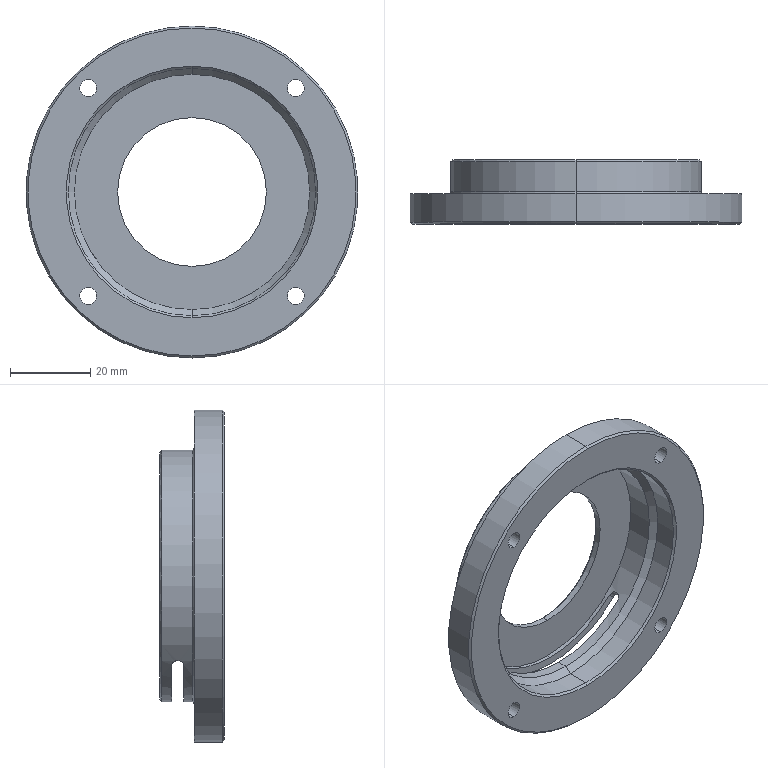Part | SolidWorks | features MoveFace 2, Chamfer 1, Fillet 1, HoleWzd 1, ICE 1, Revolution 1 | 1 solid | 56 faces | box 82.5 x 16 x 82.5 mm | volume 23486 mm3 | cylinder 30 | cone 18 | plane 6 | torus 2 | commonest cylinder face diameters 4.2 x8 8 x8 3 x4 37 x2 58.5 x2 61.5 x2